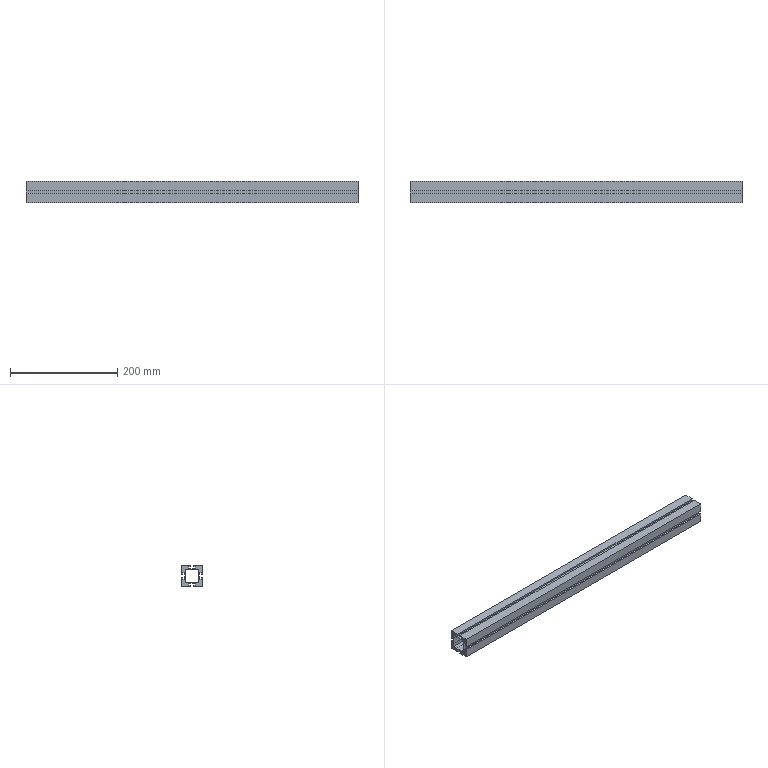Part | SolidWorks | features Extrusion 1 | 1 solid | 42 faces | box 620 x 40 x 40 mm | volume 431520 mm3 | plane 42
STEP:
#1=CARTESIAN_POINT('',(620.,3.,-20.));
#2=VERTEX_POINT('',#1);
#3=CARTESIAN_POINT('',(620.,20.,-20.));
#4=VERTEX_POINT('',#3);
#5=CARTESIAN_POINT('',(620.,3.,-20.));
#6=DIRECTION('',(0.,1.,0.));
#7=VECTOR('',#6,1000.);
#8=LINE('',#5,#7);
#9=EDGE_CURVE('',#2,#4,#8,.T.);
#10=ORIENTED_EDGE('',*,*,#9,.T.);
#11=CARTESIAN_POINT('',(620.,20.,-3.));
#12=VERTEX_POINT('',#11);
#13=CARTESIAN_POINT('',(620.,20.,-3.));
#14=DIRECTION('',(0.,0.,1.));
#15=VECTOR('',#14,1000.);
#16=LINE('',#13,#15);
#17=EDGE_CURVE('',#4,#12,#16,.T.);
#18=ORIENTED_EDGE('',*,*,#17,.T.);
#19=CARTESIAN_POINT('',(620.,17.,-3.));
#20=VERTEX_POINT('',#19);
#21=CARTESIAN_POINT('',(620.,20.,-3.));
#22=DIRECTION('',(0.,-1.,0.));
#23=VECTOR('',#22,1000.);
#24=LINE('',#21,#23);
#25=EDGE_CURVE('',#12,#20,#24,.T.);
#26=ORIENTED_EDGE('',*,*,#25,.T.);
#27=CARTESIAN_POINT('',(620.,17.,-6.5));
#28=VERTEX_POINT('',#27);
#29=CARTESIAN_POINT('',(620.,17.,-3.));
#30=DIRECTION('',(0.,0.,-1.));
#31=VECTOR('',#30,1000.);
#32=LINE('',#29,#31);
#33=EDGE_CURVE('',#20,#28,#32,.T.);
#34=ORIENTED_EDGE('',*,*,#33,.T.);
#35=CARTESIAN_POINT('',(620.,14.,-6.5));
#36=VERTEX_POINT('',#35);
#37=CARTESIAN_POINT('',(620.,17.,-6.5));
#38=DIRECTION('',(0.,-1.,0.));
#39=VECTOR('',#38,1000.);
#40=LINE('',#37,#39);
#41=EDGE_CURVE('',#28,#36,#40,.T.);
#42=ORIENTED_EDGE('',*,*,#41,.T.);
#43=CARTESIAN_POINT('',(620.,14.,6.5));
#44=VERTEX_POINT('',#43);
#45=CARTESIAN_POINT('',(620.,14.,6.5));
#46=DIRECTION('',(0.,0.,1.));
#47=VECTOR('',#46,1000.);
#48=LINE('',#45,#47);
#49=EDGE_CURVE('',#36,#44,#48,.T.);
#50=ORIENTED_EDGE('',*,*,#49,.T.);
#51=CARTESIAN_POINT('',(620.,17.,6.5));
#52=VERTEX_POINT('',#51);
#53=CARTESIAN_POINT('',(620.,17.,6.5));
#54=DIRECTION('',(0.,1.,0.));
#55=VECTOR('',#54,1000.);
#56=LINE('',#53,#55);
#57=EDGE_CURVE('',#44,#52,#56,.T.);
#58=ORIENTED_EDGE('',*,*,#57,.T.);
#59=CARTESIAN_POINT('',(620.,17.,3.));
#60=VERTEX_POINT('',#59);
#61=CARTESIAN_POINT('',(620.,17.,6.5));
#62=DIRECTION('',(0.,0.,-1.));
#63=VECTOR('',#62,1000.);
#64=LINE('',#61,#63);
#65=EDGE_CURVE('',#52,#60,#64,.T.);
#66=ORIENTED_EDGE('',*,*,#65,.T.);
#67=CARTESIAN_POINT('',(620.,20.,3.));
#68=VERTEX_POINT('',#67);
#69=CARTESIAN_POINT('',(620.,20.,3.));
#70=DIRECTION('',(0.,1.,0.));
#71=VECTOR('',#70,1000.);
#72=LINE('',#69,#71);
#73=EDGE_CURVE('',#60,#68,#72,.T.);
#74=ORIENTED_EDGE('',*,*,#73,.T.);
#75=CARTESIAN_POINT('',(620.,20.,20.));
#76=VERTEX_POINT('',#75);
#77=CARTESIAN_POINT('',(620.,20.,20.));
#78=DIRECTION('',(0.,0.,1.));
#79=VECTOR('',#78,1000.);
#80=LINE('',#77,#79);
#81=EDGE_CURVE('',#68,#76,#80,.T.);
#82=ORIENTED_EDGE('',*,*,#81,.T.);
#83=CARTESIAN_POINT('',(620.,3.,20.));
#84=VERTEX_POINT('',#83);
#85=CARTESIAN_POINT('',(620.,3.,20.));
#86=DIRECTION('',(0.,-1.,0.));
#87=VECTOR('',#86,1000.);
#88=LINE('',#85,#87);
#89=EDGE_CURVE('',#76,#84,#88,.T.);
#90=ORIENTED_EDGE('',*,*,#89,.T.);
#91=CARTESIAN_POINT('',(620.,3.,17.));
#92=VERTEX_POINT('',#91);
#93=CARTESIAN_POINT('',(620.,3.,17.));
#94=DIRECTION('',(0.,0.,-1.));
#95=VECTOR('',#94,1000.);
#96=LINE('',#93,#95);
#97=EDGE_CURVE('',#84,#92,#96,.T.);
#98=ORIENTED_EDGE('',*,*,#97,.T.);
#99=CARTESIAN_POINT('',(620.,6.5,17.));
#100=VERTEX_POINT('',#99);
#101=CARTESIAN_POINT('',(620.,3.,17.));
#102=DIRECTION('',(0.,1.,0.));
#103=VECTOR('',#102,1000.);
#104=LINE('',#101,#103);
#105=EDGE_CURVE('',#92,#100,#104,.T.);
#106=ORIENTED_EDGE('',*,*,#105,.T.);
#107=CARTESIAN_POINT('',(620.,6.5,14.));
#108=VERTEX_POINT('',#107);
#109=CARTESIAN_POINT('',(620.,6.5,14.));
#110=DIRECTION('',(0.,0.,-1.));
#111=VECTOR('',#110,1000.);
#112=LINE('',#109,#111);
#113=EDGE_CURVE('',#100,#108,#112,.T.);
#114=ORIENTED_EDGE('',*,*,#113,.T.);
#115=CARTESIAN_POINT('',(620.,-6.5,14.));
#116=VERTEX_POINT('',#115);
#117=CARTESIAN_POINT('',(620.,-6.5,14.));
#118=DIRECTION('',(0.,-1.,0.));
#119=VECTOR('',#118,1000.);
#120=LINE('',#117,#119);
#121=EDGE_CURVE('',#108,#116,#120,.T.);
#122=ORIENTED_EDGE('',*,*,#121,.T.);
#123=CARTESIAN_POINT('',(620.,-6.5,17.));
#124=VERTEX_POINT('',#123);
#125=CARTESIAN_POINT('',(620.,-6.5,14.));
#126=DIRECTION('',(0.,0.,1.));
#127=VECTOR('',#126,1000.);
#128=LINE('',#125,#127);
#129=EDGE_CURVE('',#116,#124,#128,.T.);
#130=ORIENTED_EDGE('',*,*,#129,.T.);
#131=CARTESIAN_POINT('',(620.,-3.,17.));
#132=VERTEX_POINT('',#131);
#133=CARTESIAN_POINT('',(620.,-6.5,17.));
#134=DIRECTION('',(0.,1.,0.));
#135=VECTOR('',#134,1000.);
#136=LINE('',#133,#135);
#137=EDGE_CURVE('',#124,#132,#136,.T.);
#138=ORIENTED_EDGE('',*,*,#137,.T.);
#139=CARTESIAN_POINT('',(620.,-3.,20.));
#140=VERTEX_POINT('',#139);
#141=CARTESIAN_POINT('',(620.,-3.,17.));
#142=DIRECTION('',(0.,0.,1.));
#143=VECTOR('',#142,1000.);
#144=LINE('',#141,#143);
#145=EDGE_CURVE('',#132,#140,#144,.T.);
#146=ORIENTED_EDGE('',*,*,#145,.T.);
#147=CARTESIAN_POINT('',(620.,-20.,20.));
#148=VERTEX_POINT('',#147);
#149=CARTESIAN_POINT('',(620.,-20.,20.));
#150=DIRECTION('',(0.,-1.,0.));
#151=VECTOR('',#150,1000.);
#152=LINE('',#149,#151);
#153=EDGE_CURVE('',#140,#148,#152,.T.);
#154=ORIENTED_EDGE('',*,*,#153,.T.);
#155=CARTESIAN_POINT('',(620.,-20.,3.));
#156=VERTEX_POINT('',#155);
#157=CARTESIAN_POINT('',(620.,-20.,20.));
#158=DIRECTION('',(0.,0.,-1.));
#159=VECTOR('',#158,1000.);
#160=LINE('',#157,#159);
#161=EDGE_CURVE('',#148,#156,#160,.T.);
#162=ORIENTED_EDGE('',*,*,#161,.T.);
#163=CARTESIAN_POINT('',(620.,-17.,3.));
#164=VERTEX_POINT('',#163);
#165=CARTESIAN_POINT('',(620.,-20.,3.));
#166=DIRECTION('',(0.,1.,0.));
#167=VECTOR('',#166,1000.);
#168=LINE('',#165,#167);
#169=EDGE_CURVE('',#156,#164,#168,.T.);
#170=ORIENTED_EDGE('',*,*,#169,.T.);
#171=CARTESIAN_POINT('',(620.,-17.,6.5));
#172=VERTEX_POINT('',#171);
#173=CARTESIAN_POINT('',(620.,-17.,6.5));
#174=DIRECTION('',(0.,0.,1.));
#175=VECTOR('',#174,1000.);
#176=LINE('',#173,#175);
#177=EDGE_CURVE('',#164,#172,#176,.T.);
#178=ORIENTED_EDGE('',*,*,#177,.T.);
#179=CARTESIAN_POINT('',(620.,-14.,6.5));
#180=VERTEX_POINT('',#179);
#181=CARTESIAN_POINT('',(620.,-17.,6.5));
#182=DIRECTION('',(0.,1.,0.));
#183=VECTOR('',#182,1000.);
#184=LINE('',#181,#183);
#185=EDGE_CURVE('',#172,#180,#184,.T.);
#186=ORIENTED_EDGE('',*,*,#185,.T.);
#187=CARTESIAN_POINT('',(620.,-14.,-6.5));
#188=VERTEX_POINT('',#187);
#189=CARTESIAN_POINT('',(620.,-14.,6.5));
#190=DIRECTION('',(0.,0.,-1.));
#191=VECTOR('',#190,1000.);
#192=LINE('',#189,#191);
#193=EDGE_CURVE('',#180,#188,#192,.T.);
#194=ORIENTED_EDGE('',*,*,#193,.T.);
#195=CARTESIAN_POINT('',(620.,-17.,-6.5));
#196=VERTEX_POINT('',#195);
#197=CARTESIAN_POINT('',(620.,-17.,-6.5));
#198=DIRECTION('',(0.,-1.,0.));
#199=VECTOR('',#198,1000.);
#200=LINE('',#197,#199);
#201=EDGE_CURVE('',#188,#196,#200,.T.);
#202=ORIENTED_EDGE('',*,*,#201,.T.);
#203=CARTESIAN_POINT('',(620.,-17.,-3.));
#204=VERTEX_POINT('',#203);
#205=CARTESIAN_POINT('',(620.,-17.,-3.));
#206=DIRECTION('',(0.,0.,1.));
#207=VECTOR('',#206,1000.);
#208=LINE('',#205,#207);
#209=EDGE_CURVE('',#196,#204,#208,.T.);
#210=ORIENTED_EDGE('',*,*,#209,.T.);
#211=CARTESIAN_POINT('',(620.,-20.,-3.));
#212=VERTEX_POINT('',#211);
#213=CARTESIAN_POINT('',(620.,-20.,-3.));
#214=DIRECTION('',(0.,-1.,0.));
#215=VECTOR('',#214,1000.);
#216=LINE('',#213,#215);
#217=EDGE_CURVE('',#204,#212,#216,.T.);
#218=ORIENTED_EDGE('',*,*,#217,.T.);
#219=CARTESIAN_POINT('',(620.,-20.,-20.));
#220=VERTEX_POINT('',#219);
#221=CARTESIAN_POINT('',(620.,-20.,-3.));
#222=DIRECTION('',(0.,0.,-1.));
#223=VECTOR('',#222,1000.);
#224=LINE('',#221,#223);
#225=EDGE_CURVE('',#212,#220,#224,.T.);
#226=ORIENTED_EDGE('',*,*,#225,.T.);
#227=CARTESIAN_POINT('',(620.,-3.,-20.));
#228=VERTEX_POINT('',#227);
#229=CARTESIAN_POINT('',(620.,-20.,-20.));
#230=DIRECTION('',(0.,1.,0.));
#231=VECTOR('',#230,1000.);
#232=LINE('',#229,#231);
#233=EDGE_CURVE('',#220,#228,#232,.T.);
#234=ORIENTED_EDGE('',*,*,#233,.T.);
#235=CARTESIAN_POINT('',(620.,-3.,-17.));
#236=VERTEX_POINT('',#235);
#237=CARTESIAN_POINT('',(620.,-3.,-17.));
#238=DIRECTION('',(0.,0.,1.));
#239=VECTOR('',#238,1000.);
#240=LINE('',#237,#239);
#241=EDGE_CURVE('',#228,#236,#240,.T.);
#242=ORIENTED_EDGE('',*,*,#241,.T.);
#243=CARTESIAN_POINT('',(620.,-6.5,-17.));
#244=VERTEX_POINT('',#243);
#245=CARTESIAN_POINT('',(620.,-6.5,-17.));
#246=DIRECTION('',(0.,-1.,0.));
#247=VECTOR('',#246,1000.);
#248=LINE('',#245,#247);
#249=EDGE_CURVE('',#236,#244,#248,.T.);
#250=ORIENTED_EDGE('',*,*,#249,.T.);
#251=CARTESIAN_POINT('',(620.,-6.5,-14.));
#252=VERTEX_POINT('',#251);
#253=CARTESIAN_POINT('',(620.,-6.5,-14.));
#254=DIRECTION('',(0.,0.,1.));
#255=VECTOR('',#254,1000.);
#256=LINE('',#253,#255);
#257=EDGE_CURVE('',#244,#252,#256,.T.);
#258=ORIENTED_EDGE('',*,*,#257,.T.);
#259=CARTESIAN_POINT('',(620.,6.5,-14.));
#260=VERTEX_POINT('',#259);
#261=CARTESIAN_POINT('',(620.,-6.5,-14.));
#262=DIRECTION('',(0.,1.,0.));
#263=VECTOR('',#262,1000.);
#264=LINE('',#261,#263);
#265=EDGE_CURVE('',#252,#260,#264,.T.);
#266=ORIENTED_EDGE('',*,*,#265,.T.);
#267=CARTESIAN_POINT('',(620.,6.5,-17.));
#268=VERTEX_POINT('',#267);
#269=CARTESIAN_POINT('',(620.,6.5,-14.));
#270=DIRECTION('',(0.,0.,-1.));
#271=VECTOR('',#270,1000.);
#272=LINE('',#269,#271);
#273=EDGE_CURVE('',#260,#268,#272,.T.);
#274=ORIENTED_EDGE('',*,*,#273,.T.);
#275=CARTESIAN_POINT('',(620.,3.,-17.));
#276=VERTEX_POINT('',#275);
#277=CARTESIAN_POINT('',(620.,3.,-17.));
#278=DIRECTION('',(0.,-1.,0.));
#279=VECTOR('',#278,1000.);
#280=LINE('',#277,#279);
#281=EDGE_CURVE('',#268,#276,#280,.T.);
#282=ORIENTED_EDGE('',*,*,#281,.T.);
#283=CARTESIAN_POINT('',(620.,3.,-17.));
#284=DIRECTION('',(0.,0.,-1.));
#285=VECTOR('',#284,1000.);
#286=LINE('',#283,#285);
#287=EDGE_CURVE('',#276,#2,#286,.T.);
#288=ORIENTED_EDGE('',*,*,#287,.T.);
#289=EDGE_LOOP('',(#10,#18,#26,#34,#42,#50,#58,#66,#74,#82,#90,#98,#106,#114,#122,#130,#138,#146,#154,#162,#170,#178,#186,#194,#202,#210,#218,#226,#234,#242,#250,#258,#266,#274,#282,#288));
#290=FACE_OUTER_BOUND('',#289,.T.);
#291=CARTESIAN_POINT('',(620.,-13.,-13.));
#292=VERTEX_POINT('',#291);
#293=CARTESIAN_POINT('',(620.,13.,-13.));
#294=VERTEX_POINT('',#293);
#295=CARTESIAN_POINT('',(620.,-13.,-13.));
#296=DIRECTION('',(0.,1.,0.));
#297=VECTOR('',#296,1000.);
#298=LINE('',#295,#297);
#299=EDGE_CURVE('',#292,#294,#298,.T.);
#300=ORIENTED_EDGE('',*,*,#299,.F.);
#301=CARTESIAN_POINT('',(620.,-13.,13.));
#302=VERTEX_POINT('',#301);
#303=CARTESIAN_POINT('',(620.,-13.,13.));
#304=DIRECTION('',(0.,0.,-1.));
#305=VECTOR('',#304,1000.);
#306=LINE('',#303,#305);
#307=EDGE_CURVE('',#302,#292,#306,.T.);
#308=ORIENTED_EDGE('',*,*,#307,.F.);
#309=CARTESIAN_POINT('',(620.,13.,13.));
#310=VERTEX_POINT('',#309);
#311=CARTESIAN_POINT('',(620.,-13.,13.));
#312=DIRECTION('',(0.,-1.,0.));
#313=VECTOR('',#312,1000.);
#314=LINE('',#311,#313);
#315=EDGE_CURVE('',#310,#302,#314,.T.);
#316=ORIENTED_EDGE('',*,*,#315,.F.);
#317=CARTESIAN_POINT('',(620.,13.,13.));
#318=DIRECTION('',(0.,0.,1.));
#319=VECTOR('',#318,1000.);
#320=LINE('',#317,#319);
#321=EDGE_CURVE('',#294,#310,#320,.T.);
#322=ORIENTED_EDGE('',*,*,#321,.F.);
#323=EDGE_LOOP('',(#300,#308,#316,#322));
#324=FACE_BOUND('',#323,.T.);
#325=CARTESIAN_POINT('',(620.,20.,-20.));
#326=DIRECTION('',(-1.,0.,0.));
#327=DIRECTION('',(0.,0.,1.));
#328=AXIS2_PLACEMENT_3D('',#325,#326,#327);
#329=PLANE('',#328);
#330=ADVANCED_FACE('',(#290,#324),#329,.F.);
#331=CARTESIAN_POINT('',(0.,3.,-20.));
#332=VERTEX_POINT('',#331);
#333=CARTESIAN_POINT('',(0.,20.,-20.));
#334=VERTEX_POINT('',#333);
#335=CARTESIAN_POINT('',(0.,3.,-20.));
#336=DIRECTION('',(0.,1.,0.));
#337=VECTOR('',#336,1000.);
#338=LINE('',#335,#337);
#339=EDGE_CURVE('',#332,#334,#338,.T.);
#340=ORIENTED_EDGE('',*,*,#339,.F.);
#341=CARTESIAN_POINT('',(0.,3.,-17.));
#342=VERTEX_POINT('',#341);
#343=CARTESIAN_POINT('',(0.,3.,-17.));
#344=DIRECTION('',(0.,0.,-1.));
#345=VECTOR('',#344,1000.);
#346=LINE('',#343,#345);
#347=EDGE_CURVE('',#342,#332,#346,.T.);
#348=ORIENTED_EDGE('',*,*,#347,.F.);
#349=CARTESIAN_POINT('',(0.,6.5,-17.));
#350=VERTEX_POINT('',#349);
#351=CARTESIAN_POINT('',(0.,3.,-17.));
#352=DIRECTION('',(0.,-1.,0.));
#353=VECTOR('',#352,1000.);
#354=LINE('',#351,#353);
#355=EDGE_CURVE('',#350,#342,#354,.T.);
#356=ORIENTED_EDGE('',*,*,#355,.F.);
#357=CARTESIAN_POINT('',(0.,6.5,-14.));
#358=VERTEX_POINT('',#357);
#359=CARTESIAN_POINT('',(0.,6.5,-14.));
#360=DIRECTION('',(0.,0.,-1.));
#361=VECTOR('',#360,1000.);
#362=LINE('',#359,#361);
#363=EDGE_CURVE('',#358,#350,#362,.T.);
#364=ORIENTED_EDGE('',*,*,#363,.F.);
#365=CARTESIAN_POINT('',(0.,-6.5,-14.));
#366=VERTEX_POINT('',#365);
#367=CARTESIAN_POINT('',(0.,-6.5,-14.));
#368=DIRECTION('',(0.,1.,0.));
#369=VECTOR('',#368,1000.);
#370=LINE('',#367,#369);
#371=EDGE_CURVE('',#366,#358,#370,.T.);
#372=ORIENTED_EDGE('',*,*,#371,.F.);
#373=CARTESIAN_POINT('',(0.,-6.5,-17.));
#374=VERTEX_POINT('',#373);
#375=CARTESIAN_POINT('',(0.,-6.5,-14.));
#376=DIRECTION('',(0.,0.,1.));
#377=VECTOR('',#376,1000.);
#378=LINE('',#375,#377);
#379=EDGE_CURVE('',#374,#366,#378,.T.);
#380=ORIENTED_EDGE('',*,*,#379,.F.);
#381=CARTESIAN_POINT('',(0.,-3.,-17.));
#382=VERTEX_POINT('',#381);
#383=CARTESIAN_POINT('',(0.,-6.5,-17.));
#384=DIRECTION('',(0.,-1.,0.));
#385=VECTOR('',#384,1000.);
#386=LINE('',#383,#385);
#387=EDGE_CURVE('',#382,#374,#386,.T.);
#388=ORIENTED_EDGE('',*,*,#387,.F.);
#389=CARTESIAN_POINT('',(0.,-3.,-20.));
#390=VERTEX_POINT('',#389);
#391=CARTESIAN_POINT('',(0.,-3.,-17.));
#392=DIRECTION('',(0.,0.,1.));
#393=VECTOR('',#392,1000.);
#394=LINE('',#391,#393);
#395=EDGE_CURVE('',#390,#382,#394,.T.);
#396=ORIENTED_EDGE('',*,*,#395,.F.);
#397=CARTESIAN_POINT('',(0.,-20.,-20.));
#398=VERTEX_POINT('',#397);
#399=CARTESIAN_POINT('',(0.,-20.,-20.));
#400=DIRECTION('',(0.,1.,0.));
#401=VECTOR('',#400,1000.);
#402=LINE('',#399,#401);
#403=EDGE_CURVE('',#398,#390,#402,.T.);
#404=ORIENTED_EDGE('',*,*,#403,.F.);
#405=CARTESIAN_POINT('',(0.,-20.,-3.));
#406=VERTEX_POINT('',#405);
#407=CARTESIAN_POINT('',(0.,-20.,-3.));
#408=DIRECTION('',(0.,0.,-1.));
#409=VECTOR('',#408,1000.);
#410=LINE('',#407,#409);
#411=EDGE_CURVE('',#406,#398,#410,.T.);
#412=ORIENTED_EDGE('',*,*,#411,.F.);
#413=CARTESIAN_POINT('',(0.,-17.,-3.));
#414=VERTEX_POINT('',#413);
#415=CARTESIAN_POINT('',(0.,-20.,-3.));
#416=DIRECTION('',(0.,-1.,0.));
#417=VECTOR('',#416,1000.);
#418=LINE('',#415,#417);
#419=EDGE_CURVE('',#414,#406,#418,.T.);
#420=ORIENTED_EDGE('',*,*,#419,.F.);
#421=CARTESIAN_POINT('',(0.,-17.,-6.5));
#422=VERTEX_POINT('',#421);
#423=CARTESIAN_POINT('',(0.,-17.,-3.));
#424=DIRECTION('',(0.,0.,1.));
#425=VECTOR('',#424,1000.);
#426=LINE('',#423,#425);
#427=EDGE_CURVE('',#422,#414,#426,.T.);
#428=ORIENTED_EDGE('',*,*,#427,.F.);
#429=CARTESIAN_POINT('',(0.,-14.,-6.5));
#430=VERTEX_POINT('',#429);
#431=CARTESIAN_POINT('',(0.,-17.,-6.5));
#432=DIRECTION('',(0.,-1.,0.));
#433=VECTOR('',#432,1000.);
#434=LINE('',#431,#433);
#435=EDGE_CURVE('',#430,#422,#434,.T.);
#436=ORIENTED_EDGE('',*,*,#435,.F.);
#437=CARTESIAN_POINT('',(0.,-14.,6.5));
#438=VERTEX_POINT('',#437);
#439=CARTESIAN_POINT('',(0.,-14.,6.5));
#440=DIRECTION('',(0.,0.,-1.));
#441=VECTOR('',#440,1000.);
#442=LINE('',#439,#441);
#443=EDGE_CURVE('',#438,#430,#442,.T.);
#444=ORIENTED_EDGE('',*,*,#443,.F.);
#445=CARTESIAN_POINT('',(0.,-17.,6.5));
#446=VERTEX_POINT('',#445);
#447=CARTESIAN_POINT('',(0.,-17.,6.5));
#448=DIRECTION('',(0.,1.,0.));
#449=VECTOR('',#448,1000.);
#450=LINE('',#447,#449);
#451=EDGE_CURVE('',#446,#438,#450,.T.);
#452=ORIENTED_EDGE('',*,*,#451,.F.);
#453=CARTESIAN_POINT('',(0.,-17.,3.));
#454=VERTEX_POINT('',#453);
#455=CARTESIAN_POINT('',(0.,-17.,6.5));
#456=DIRECTION('',(0.,0.,1.));
#457=VECTOR('',#456,1000.);
#458=LINE('',#455,#457);
#459=EDGE_CURVE('',#454,#446,#458,.T.);
#460=ORIENTED_EDGE('',*,*,#459,.F.);
#461=CARTESIAN_POINT('',(0.,-20.,3.));
#462=VERTEX_POINT('',#461);
#463=CARTESIAN_POINT('',(0.,-20.,3.));
#464=DIRECTION('',(0.,1.,0.));
#465=VECTOR('',#464,1000.);
#466=LINE('',#463,#465);
#467=EDGE_CURVE('',#462,#454,#466,.T.);
#468=ORIENTED_EDGE('',*,*,#467,.F.);
#469=CARTESIAN_POINT('',(0.,-20.,20.));
#470=VERTEX_POINT('',#469);
#471=CARTESIAN_POINT('',(0.,-20.,20.));
#472=DIRECTION('',(0.,0.,-1.));
#473=VECTOR('',#472,1000.);
#474=LINE('',#471,#473);
#475=EDGE_CURVE('',#470,#462,#474,.T.);
#476=ORIENTED_EDGE('',*,*,#475,.F.);
#477=CARTESIAN_POINT('',(0.,-3.,20.));
#478=VERTEX_POINT('',#477);
#479=CARTESIAN_POINT('',(0.,-20.,20.));
#480=DIRECTION('',(0.,-1.,0.));
#481=VECTOR('',#480,1000.);
#482=LINE('',#479,#481);
#483=EDGE_CURVE('',#478,#470,#482,.T.);
#484=ORIENTED_EDGE('',*,*,#483,.F.);
#485=CARTESIAN_POINT('',(0.,-3.,17.));
#486=VERTEX_POINT('',#485);
#487=CARTESIAN_POINT('',(0.,-3.,17.));
#488=DIRECTION('',(0.,0.,1.));
#489=VECTOR('',#488,1000.);
#490=LINE('',#487,#489);
#491=EDGE_CURVE('',#486,#478,#490,.T.);
#492=ORIENTED_EDGE('',*,*,#491,.F.);
#493=CARTESIAN_POINT('',(0.,-6.5,17.));
#494=VERTEX_POINT('',#493);
#495=CARTESIAN_POINT('',(0.,-6.5,17.));
#496=DIRECTION('',(0.,1.,0.));
#497=VECTOR('',#496,1000.);
#498=LINE('',#495,#497);
#499=EDGE_CURVE('',#494,#486,#498,.T.);
#500=ORIENTED_EDGE('',*,*,#499,.F.);
#501=CARTESIAN_POINT('',(0.,-6.5,14.));
#502=VERTEX_POINT('',#501);
#503=CARTESIAN_POINT('',(0.,-6.5,14.));
#504=DIRECTION('',(0.,0.,1.));
#505=VECTOR('',#504,1000.);
#506=LINE('',#503,#505);
#507=EDGE_CURVE('',#502,#494,#506,.T.);
#508=ORIENTED_EDGE('',*,*,#507,.F.);
#509=CARTESIAN_POINT('',(0.,6.5,14.));
#510=VERTEX_POINT('',#509);
#511=CARTESIAN_POINT('',(0.,-6.5,14.));
#512=DIRECTION('',(0.,-1.,0.));
#513=VECTOR('',#512,1000.);
#514=LINE('',#511,#513);
#515=EDGE_CURVE('',#510,#502,#514,.T.);
#516=ORIENTED_EDGE('',*,*,#515,.F.);
#517=CARTESIAN_POINT('',(0.,6.5,17.));
#518=VERTEX_POINT('',#517);
#519=CARTESIAN_POINT('',(0.,6.5,14.));
#520=DIRECTION('',(0.,0.,-1.));
#521=VECTOR('',#520,1000.);
#522=LINE('',#519,#521);
#523=EDGE_CURVE('',#518,#510,#522,.T.);
#524=ORIENTED_EDGE('',*,*,#523,.F.);
#525=CARTESIAN_POINT('',(0.,3.,17.));
#526=VERTEX_POINT('',#525);
#527=CARTESIAN_POINT('',(0.,3.,17.));
#528=DIRECTION('',(0.,1.,0.));
#529=VECTOR('',#528,1000.);
#530=LINE('',#527,#529);
#531=EDGE_CURVE('',#526,#518,#530,.T.);
#532=ORIENTED_EDGE('',*,*,#531,.F.);
#533=CARTESIAN_POINT('',(0.,3.,20.));
#534=VERTEX_POINT('',#533);
#535=CARTESIAN_POINT('',(0.,3.,17.));
#536=DIRECTION('',(0.,0.,-1.));
#537=VECTOR('',#536,1000.);
#538=LINE('',#535,#537);
#539=EDGE_CURVE('',#534,#526,#538,.T.);
#540=ORIENTED_EDGE('',*,*,#539,.F.);
#541=CARTESIAN_POINT('',(0.,20.,20.));
#542=VERTEX_POINT('',#541);
#543=CARTESIAN_POINT('',(0.,3.,20.));
#544=DIRECTION('',(0.,-1.,0.));
#545=VECTOR('',#544,1000.);
#546=LINE('',#543,#545);
#547=EDGE_CURVE('',#542,#534,#546,.T.);
#548=ORIENTED_EDGE('',*,*,#547,.F.);
#549=CARTESIAN_POINT('',(0.,20.,3.));
#550=VERTEX_POINT('',#549);
#551=CARTESIAN_POINT('',(0.,20.,20.));
#552=DIRECTION('',(0.,0.,1.));
#553=VECTOR('',#552,1000.);
#554=LINE('',#551,#553);
#555=EDGE_CURVE('',#550,#542,#554,.T.);
#556=ORIENTED_EDGE('',*,*,#555,.F.);
#557=CARTESIAN_POINT('',(0.,17.,3.));
#558=VERTEX_POINT('',#557);
#559=CARTESIAN_POINT('',(0.,20.,3.));
#560=DIRECTION('',(0.,1.,0.));
#561=VECTOR('',#560,1000.);
#562=LINE('',#559,#561);
#563=EDGE_CURVE('',#558,#550,#562,.T.);
#564=ORIENTED_EDGE('',*,*,#563,.F.);
#565=CARTESIAN_POINT('',(0.,17.,6.5));
#566=VERTEX_POINT('',#565);
#567=CARTESIAN_POINT('',(0.,17.,6.5));
#568=DIRECTION('',(0.,0.,-1.));
#569=VECTOR('',#568,1000.);
#570=LINE('',#567,#569);
#571=EDGE_CURVE('',#566,#558,#570,.T.);
#572=ORIENTED_EDGE('',*,*,#571,.F.);
#573=CARTESIAN_POINT('',(0.,14.,6.5));
#574=VERTEX_POINT('',#573);
#575=CARTESIAN_POINT('',(0.,17.,6.5));
#576=DIRECTION('',(0.,1.,0.));
#577=VECTOR('',#576,1000.);
#578=LINE('',#575,#577);
#579=EDGE_CURVE('',#574,#566,#578,.T.);
#580=ORIENTED_EDGE('',*,*,#579,.F.);
#581=CARTESIAN_POINT('',(0.,14.,-6.5));
#582=VERTEX_POINT('',#581);
#583=CARTESIAN_POINT('',(0.,14.,6.5));
#584=DIRECTION('',(0.,0.,1.));
#585=VECTOR('',#584,1000.);
#586=LINE('',#583,#585);
#587=EDGE_CURVE('',#582,#574,#586,.T.);
#588=ORIENTED_EDGE('',*,*,#587,.F.);
#589=CARTESIAN_POINT('',(0.,17.,-6.5));
#590=VERTEX_POINT('',#589);
#591=CARTESIAN_POINT('',(0.,17.,-6.5));
#592=DIRECTION('',(0.,-1.,0.));
#593=VECTOR('',#592,1000.);
#594=LINE('',#591,#593);
#595=EDGE_CURVE('',#590,#582,#594,.T.);
#596=ORIENTED_EDGE('',*,*,#595,.F.);
#597=CARTESIAN_POINT('',(0.,17.,-3.));
#598=VERTEX_POINT('',#597);
#599=CARTESIAN_POINT('',(0.,17.,-3.));
#600=DIRECTION('',(0.,0.,-1.));
#601=VECTOR('',#600,1000.);
#602=LINE('',#599,#601);
#603=EDGE_CURVE('',#598,#590,#602,.T.);
#604=ORIENTED_EDGE('',*,*,#603,.F.);
#605=CARTESIAN_POINT('',(0.,20.,-3.));
#606=VERTEX_POINT('',#605);
#607=CARTESIAN_POINT('',(0.,20.,-3.));
#608=DIRECTION('',(0.,-1.,0.));
#609=VECTOR('',#608,1000.);
#610=LINE('',#607,#609);
#611=EDGE_CURVE('',#606,#598,#610,.T.);
#612=ORIENTED_EDGE('',*,*,#611,.F.);
#613=CARTESIAN_POINT('',(0.,20.,-3.));
#614=DIRECTION('',(0.,0.,1.));
#615=VECTOR('',#614,1000.);
#616=LINE('',#613,#615);
#617=EDGE_CURVE('',#334,#606,#616,.T.);
#618=ORIENTED_EDGE('',*,*,#617,.F.);
#619=EDGE_LOOP('',(#340,#348,#356,#364,#372,#380,#388,#396,#404,#412,#420,#428,#436,#444,#452,#460,#468,#476,#484,#492,#500,#508,#516,#524,#532,#540,#548,#556,#564,#572,#580,#588,#596,#604,#612,#618));
#620=FACE_OUTER_BOUND('',#619,.T.);
#621=CARTESIAN_POINT('',(0.,-13.,13.));
#622=VERTEX_POINT('',#621);
#623=CARTESIAN_POINT('',(0.,-13.,-13.));
#624=VERTEX_POINT('',#623);
#625=CARTESIAN_POINT('',(0.,-13.,13.));
#626=DIRECTION('',(0.,0.,-1.));
#627=VECTOR('',#626,1000.);
#628=LINE('',#625,#627);
#629=EDGE_CURVE('',#622,#624,#628,.T.);
#630=ORIENTED_EDGE('',*,*,#629,.T.);
#631=CARTESIAN_POINT('',(0.,13.,-13.));
#632=VERTEX_POINT('',#631);
#633=CARTESIAN_POINT('',(0.,-13.,-13.));
#634=DIRECTION('',(0.,1.,0.));
#635=VECTOR('',#634,1000.);
#636=LINE('',#633,#635);
#637=EDGE_CURVE('',#624,#632,#636,.T.);
#638=ORIENTED_EDGE('',*,*,#637,.T.);
#639=CARTESIAN_POINT('',(0.,13.,13.));
#640=VERTEX_POINT('',#639);
#641=CARTESIAN_POINT('',(0.,13.,13.));
#642=DIRECTION('',(0.,0.,1.));
#643=VECTOR('',#642,1000.);
#644=LINE('',#641,#643);
#645=EDGE_CURVE('',#632,#640,#644,.T.);
#646=ORIENTED_EDGE('',*,*,#645,.T.);
#647=CARTESIAN_POINT('',(0.,-13.,13.));
#648=DIRECTION('',(0.,-1.,0.));
#649=VECTOR('',#648,1000.);
#650=LINE('',#647,#649);
#651=EDGE_CURVE('',#640,#622,#650,.T.);
#652=ORIENTED_EDGE('',*,*,#651,.T.);
#653=EDGE_LOOP('',(#630,#638,#646,#652));
#654=FACE_BOUND('',#653,.T.);
#655=CARTESIAN_POINT('',(0.,20.,-20.));
#656=DIRECTION('',(-1.,0.,0.));
#657=DIRECTION('',(0.,0.,1.));
#658=AXIS2_PLACEMENT_3D('',#655,#656,#657);
#659=PLANE('',#658);
#660=ADVANCED_FACE('',(#620,#654),#659,.T.);
#661=ORIENTED_EDGE('',*,*,#339,.T.);
#662=CARTESIAN_POINT('',(620.,20.,-20.));
#663=DIRECTION('',(-1.,0.,0.));
#664=VECTOR('',#663,1000.);
#665=LINE('',#662,#664);
#666=EDGE_CURVE('',#4,#334,#665,.T.);
#667=ORIENTED_EDGE('',*,*,#666,.F.);
#668=ORIENTED_EDGE('',*,*,#9,.F.);
#669=CARTESIAN_POINT('',(620.,3.,-20.));
#670=DIRECTION('',(-1.,0.,0.));
#671=VECTOR('',#670,1000.);
#672=LINE('',#669,#671);
#673=EDGE_CURVE('',#2,#332,#672,.T.);
#674=ORIENTED_EDGE('',*,*,#673,.T.);
#675=EDGE_LOOP('',(#661,#667,#668,#674));
#676=FACE_OUTER_BOUND('',#675,.T.);
#677=CARTESIAN_POINT('',(620.,3.,-20.));
#678=DIRECTION('',(0.,0.,1.));
#679=DIRECTION('',(0.,-1.,0.));
#680=AXIS2_PLACEMENT_3D('',#677,#678,#679);
#681=PLANE('',#680);
#682=ADVANCED_FACE('',(#676),#681,.F.);
#683=ORIENTED_EDGE('',*,*,#617,.T.);
#684=CARTESIAN_POINT('',(620.,20.,-3.));
#685=DIRECTION('',(-1.,0.,0.));
#686=VECTOR('',#685,1000.);
#687=LINE('',#684,#686);
#688=EDGE_CURVE('',#12,#606,#687,.T.);
#689=ORIENTED_EDGE('',*,*,#688,.F.);
#690=ORIENTED_EDGE('',*,*,#17,.F.);
#691=ORIENTED_EDGE('',*,*,#666,.T.);
#692=EDGE_LOOP('',(#683,#689,#690,#691));
#693=FACE_OUTER_BOUND('',#692,.T.);
#694=CARTESIAN_POINT('',(620.,20.,-3.));
#695=DIRECTION('',(0.,-1.,0.));
#696=DIRECTION('',(0.,0.,-1.));
#697=AXIS2_PLACEMENT_3D('',#694,#695,#696);
#698=PLANE('',#697);
#699=ADVANCED_FACE('',(#693),#698,.F.);
#700=ORIENTED_EDGE('',*,*,#611,.T.);
#701=CARTESIAN_POINT('',(620.,17.,-3.));
#702=DIRECTION('',(-1.,0.,0.));
#703=VECTOR('',#702,1000.);
#704=LINE('',#701,#703);
#705=EDGE_CURVE('',#20,#598,#704,.T.);
#706=ORIENTED_EDGE('',*,*,#705,.F.);
#707=ORIENTED_EDGE('',*,*,#25,.F.);
#708=ORIENTED_EDGE('',*,*,#688,.T.);
#709=EDGE_LOOP('',(#700,#706,#707,#708));
#710=FACE_OUTER_BOUND('',#709,.T.);
#711=CARTESIAN_POINT('',(620.,20.,-3.));
#712=DIRECTION('',(0.,0.,-1.));
#713=DIRECTION('',(0.,1.,0.));
#714=AXIS2_PLACEMENT_3D('',#711,#712,#713);
#715=PLANE('',#714);
#716=ADVANCED_FACE('',(#710),#715,.F.);
#717=ORIENTED_EDGE('',*,*,#603,.T.);
#718=CARTESIAN_POINT('',(620.,17.,-6.5));
#719=DIRECTION('',(-1.,0.,0.));
#720=VECTOR('',#719,1000.);
#721=LINE('',#718,#720);
#722=EDGE_CURVE('',#28,#590,#721,.T.);
#723=ORIENTED_EDGE('',*,*,#722,.F.);
#724=ORIENTED_EDGE('',*,*,#33,.F.);
#725=ORIENTED_EDGE('',*,*,#705,.T.);
#726=EDGE_LOOP('',(#717,#723,#724,#725));
#727=FACE_OUTER_BOUND('',#726,.T.);
#728=CARTESIAN_POINT('',(620.,17.,-3.));
#729=DIRECTION('',(0.,1.,0.));
#730=DIRECTION('',(0.,0.,1.));
#731=AXIS2_PLACEMENT_3D('',#728,#729,#730);
#732=PLANE('',#731);
#733=ADVANCED_FACE('',(#727),#732,.F.);
#734=ORIENTED_EDGE('',*,*,#595,.T.);
#735=CARTESIAN_POINT('',(620.,14.,-6.5));
#736=DIRECTION('',(-1.,0.,0.));
#737=VECTOR('',#736,1000.);
#738=LINE('',#735,#737);
#739=EDGE_CURVE('',#36,#582,#738,.T.);
#740=ORIENTED_EDGE('',*,*,#739,.F.);
#741=ORIENTED_EDGE('',*,*,#41,.F.);
#742=ORIENTED_EDGE('',*,*,#722,.T.);
#743=EDGE_LOOP('',(#734,#740,#741,#742));
#744=FACE_OUTER_BOUND('',#743,.T.);
#745=CARTESIAN_POINT('',(620.,17.,-6.5));
#746=DIRECTION('',(0.,0.,-1.));
#747=DIRECTION('',(-1.,0.,0.));
#748=AXIS2_PLACEMENT_3D('',#745,#746,#747);
#749=PLANE('',#748);
#750=ADVANCED_FACE('',(#744),#749,.F.);
#751=ORIENTED_EDGE('',*,*,#587,.T.);
#752=CARTESIAN_POINT('',(620.,14.,6.5));
#753=DIRECTION('',(-1.,0.,0.));
#754=VECTOR('',#753,1000.);
#755=LINE('',#752,#754);
#756=EDGE_CURVE('',#44,#574,#755,.T.);
#757=ORIENTED_EDGE('',*,*,#756,.F.);
#758=ORIENTED_EDGE('',*,*,#49,.F.);
#759=ORIENTED_EDGE('',*,*,#739,.T.);
#760=EDGE_LOOP('',(#751,#757,#758,#759));
#761=FACE_OUTER_BOUND('',#760,.T.);
#762=CARTESIAN_POINT('',(620.,14.,6.5));
#763=DIRECTION('',(0.,-1.,0.));
#764=DIRECTION('',(0.,0.,-1.));
#765=AXIS2_PLACEMENT_3D('',#762,#763,#764);
#766=PLANE('',#765);
#767=ADVANCED_FACE('',(#761),#766,.F.);
#768=ORIENTED_EDGE('',*,*,#579,.T.);
#769=CARTESIAN_POINT('',(620.,17.,6.5));
#770=DIRECTION('',(-1.,0.,0.));
#771=VECTOR('',#770,1000.);
#772=LINE('',#769,#771);
#773=EDGE_CURVE('',#52,#566,#772,.T.);
#774=ORIENTED_EDGE('',*,*,#773,.F.);
#775=ORIENTED_EDGE('',*,*,#57,.F.);
#776=ORIENTED_EDGE('',*,*,#756,.T.);
#777=EDGE_LOOP('',(#768,#774,#775,#776));
#778=FACE_OUTER_BOUND('',#777,.T.);
#779=CARTESIAN_POINT('',(620.,17.,6.5));
#780=DIRECTION('',(0.,0.,1.));
#781=DIRECTION('',(1.,0.,0.));
#782=AXIS2_PLACEMENT_3D('',#779,#780,#781);
#783=PLANE('',#782);
#784=ADVANCED_FACE('',(#778),#783,.F.);
#785=ORIENTED_EDGE('',*,*,#571,.T.);
#786=CARTESIAN_POINT('',(620.,17.,3.));
#787=DIRECTION('',(-1.,0.,0.));
#788=VECTOR('',#787,1000.);
#789=LINE('',#786,#788);
#790=EDGE_CURVE('',#60,#558,#789,.T.);
#791=ORIENTED_EDGE('',*,*,#790,.F.);
#792=ORIENTED_EDGE('',*,*,#65,.F.);
#793=ORIENTED_EDGE('',*,*,#773,.T.);
#794=EDGE_LOOP('',(#785,#791,#792,#793));
#795=FACE_OUTER_BOUND('',#794,.T.);
#796=CARTESIAN_POINT('',(620.,17.,6.5));
#797=DIRECTION('',(0.,1.,0.));
#798=DIRECTION('',(0.,0.,1.));
#799=AXIS2_PLACEMENT_3D('',#796,#797,#798);
#800=PLANE('',#799);
#801=ADVANCED_FACE('',(#795),#800,.F.);
#802=ORIENTED_EDGE('',*,*,#563,.T.);
#803=CARTESIAN_POINT('',(620.,20.,3.));
#804=DIRECTION('',(-1.,0.,0.));
#805=VECTOR('',#804,1000.);
#806=LINE('',#803,#805);
#807=EDGE_CURVE('',#68,#550,#806,.T.);
#808=ORIENTED_EDGE('',*,*,#807,.F.);
#809=ORIENTED_EDGE('',*,*,#73,.F.);
#810=ORIENTED_EDGE('',*,*,#790,.T.);
#811=EDGE_LOOP('',(#802,#808,#809,#810));
#812=FACE_OUTER_BOUND('',#811,.T.);
#813=CARTESIAN_POINT('',(620.,20.,3.));
#814=DIRECTION('',(0.,0.,1.));
#815=DIRECTION('',(0.,-1.,0.));
#816=AXIS2_PLACEMENT_3D('',#813,#814,#815);
#817=PLANE('',#816);
#818=ADVANCED_FACE('',(#812),#817,.F.);
#819=ORIENTED_EDGE('',*,*,#555,.T.);
#820=CARTESIAN_POINT('',(620.,20.,20.));
#821=DIRECTION('',(-1.,0.,0.));
#822=VECTOR('',#821,1000.);
#823=LINE('',#820,#822);
#824=EDGE_CURVE('',#76,#542,#823,.T.);
#825=ORIENTED_EDGE('',*,*,#824,.F.);
#826=ORIENTED_EDGE('',*,*,#81,.F.);
#827=ORIENTED_EDGE('',*,*,#807,.T.);
#828=EDGE_LOOP('',(#819,#825,#826,#827));
#829=FACE_OUTER_BOUND('',#828,.T.);
#830=CARTESIAN_POINT('',(620.,20.,20.));
#831=DIRECTION('',(0.,-1.,0.));
#832=DIRECTION('',(0.,0.,-1.));
#833=AXIS2_PLACEMENT_3D('',#830,#831,#832);
#834=PLANE('',#833);
#835=ADVANCED_FACE('',(#829),#834,.F.);
#836=ORIENTED_EDGE('',*,*,#547,.T.);
#837=CARTESIAN_POINT('',(620.,3.,20.));
#838=DIRECTION('',(-1.,0.,0.));
#839=VECTOR('',#838,1000.);
#840=LINE('',#837,#839);
#841=EDGE_CURVE('',#84,#534,#840,.T.);
#842=ORIENTED_EDGE('',*,*,#841,.F.);
#843=ORIENTED_EDGE('',*,*,#89,.F.);
#844=ORIENTED_EDGE('',*,*,#824,.T.);
#845=EDGE_LOOP('',(#836,#842,#843,#844));
#846=FACE_OUTER_BOUND('',#845,.T.);
#847=CARTESIAN_POINT('',(620.,3.,20.));
#848=DIRECTION('',(0.,0.,-1.));
#849=DIRECTION('',(0.,1.,0.));
#850=AXIS2_PLACEMENT_3D('',#847,#848,#849);
#851=PLANE('',#850);
#852=ADVANCED_FACE('',(#846),#851,.F.);
#853=ORIENTED_EDGE('',*,*,#539,.T.);
#854=CARTESIAN_POINT('',(620.,3.,17.));
#855=DIRECTION('',(-1.,0.,0.));
#856=VECTOR('',#855,1000.);
#857=LINE('',#854,#856);
#858=EDGE_CURVE('',#92,#526,#857,.T.);
#859=ORIENTED_EDGE('',*,*,#858,.F.);
#860=ORIENTED_EDGE('',*,*,#97,.F.);
#861=ORIENTED_EDGE('',*,*,#841,.T.);
#862=EDGE_LOOP('',(#853,#859,#860,#861));
#863=FACE_OUTER_BOUND('',#862,.T.);
#864=CARTESIAN_POINT('',(620.,3.,17.));
#865=DIRECTION('',(0.,1.,0.));
#866=DIRECTION('',(0.,0.,1.));
#867=AXIS2_PLACEMENT_3D('',#864,#865,#866);
#868=PLANE('',#867);
#869=ADVANCED_FACE('',(#863),#868,.F.);
#870=ORIENTED_EDGE('',*,*,#531,.T.);
#871=CARTESIAN_POINT('',(620.,6.5,17.));
#872=DIRECTION('',(-1.,0.,0.));
#873=VECTOR('',#872,1000.);
#874=LINE('',#871,#873);
#875=EDGE_CURVE('',#100,#518,#874,.T.);
#876=ORIENTED_EDGE('',*,*,#875,.F.);
#877=ORIENTED_EDGE('',*,*,#105,.F.);
#878=ORIENTED_EDGE('',*,*,#858,.T.);
#879=EDGE_LOOP('',(#870,#876,#877,#878));
#880=FACE_OUTER_BOUND('',#879,.T.);
#881=CARTESIAN_POINT('',(620.,3.,17.));
#882=DIRECTION('',(0.,0.,1.));
#883=DIRECTION('',(1.,0.,0.));
#884=AXIS2_PLACEMENT_3D('',#881,#882,#883);
#885=PLANE('',#884);
#886=ADVANCED_FACE('',(#880),#885,.F.);
#887=ORIENTED_EDGE('',*,*,#523,.T.);
#888=CARTESIAN_POINT('',(620.,6.5,14.));
#889=DIRECTION('',(-1.,0.,0.));
#890=VECTOR('',#889,1000.);
#891=LINE('',#888,#890);
#892=EDGE_CURVE('',#108,#510,#891,.T.);
#893=ORIENTED_EDGE('',*,*,#892,.F.);
#894=ORIENTED_EDGE('',*,*,#113,.F.);
#895=ORIENTED_EDGE('',*,*,#875,.T.);
#896=EDGE_LOOP('',(#887,#893,#894,#895));
#897=FACE_OUTER_BOUND('',#896,.T.);
#898=CARTESIAN_POINT('',(620.,6.5,14.));
#899=DIRECTION('',(0.,1.,0.));
#900=DIRECTION('',(0.,0.,1.));
#901=AXIS2_PLACEMENT_3D('',#898,#899,#900);
#902=PLANE('',#901);
#903=ADVANCED_FACE('',(#897),#902,.F.);
#904=ORIENTED_EDGE('',*,*,#515,.T.);
#905=CARTESIAN_POINT('',(620.,-6.5,14.));
#906=DIRECTION('',(-1.,0.,0.));
#907=VECTOR('',#906,1000.);
#908=LINE('',#905,#907);
#909=EDGE_CURVE('',#116,#502,#908,.T.);
#910=ORIENTED_EDGE('',*,*,#909,.F.);
#911=ORIENTED_EDGE('',*,*,#121,.F.);
#912=ORIENTED_EDGE('',*,*,#892,.T.);
#913=EDGE_LOOP('',(#904,#910,#911,#912));
#914=FACE_OUTER_BOUND('',#913,.T.);
#915=CARTESIAN_POINT('',(620.,-6.5,14.));
#916=DIRECTION('',(0.,0.,-1.));
#917=DIRECTION('',(-1.,0.,0.));
#918=AXIS2_PLACEMENT_3D('',#915,#916,#917);
#919=PLANE('',#918);
#920=ADVANCED_FACE('',(#914),#919,.F.);
#921=ORIENTED_EDGE('',*,*,#507,.T.);
#922=CARTESIAN_POINT('',(620.,-6.5,17.));
#923=DIRECTION('',(-1.,0.,0.));
#924=VECTOR('',#923,1000.);
#925=LINE('',#922,#924);
#926=EDGE_CURVE('',#124,#494,#925,.T.);
#927=ORIENTED_EDGE('',*,*,#926,.F.);
#928=ORIENTED_EDGE('',*,*,#129,.F.);
#929=ORIENTED_EDGE('',*,*,#909,.T.);
#930=EDGE_LOOP('',(#921,#927,#928,#929));
#931=FACE_OUTER_BOUND('',#930,.T.);
#932=CARTESIAN_POINT('',(620.,-6.5,14.));
#933=DIRECTION('',(0.,-1.,0.));
#934=DIRECTION('',(0.,0.,-1.));
#935=AXIS2_PLACEMENT_3D('',#932,#933,#934);
#936=PLANE('',#935);
#937=ADVANCED_FACE('',(#931),#936,.F.);
#938=ORIENTED_EDGE('',*,*,#499,.T.);
#939=CARTESIAN_POINT('',(620.,-3.,17.));
#940=DIRECTION('',(-1.,0.,0.));
#941=VECTOR('',#940,1000.);
#942=LINE('',#939,#941);
#943=EDGE_CURVE('',#132,#486,#942,.T.);
#944=ORIENTED_EDGE('',*,*,#943,.F.);
#945=ORIENTED_EDGE('',*,*,#137,.F.);
#946=ORIENTED_EDGE('',*,*,#926,.T.);
#947=EDGE_LOOP('',(#938,#944,#945,#946));
#948=FACE_OUTER_BOUND('',#947,.T.);
#949=CARTESIAN_POINT('',(620.,-6.5,17.));
#950=DIRECTION('',(0.,0.,1.));
#951=DIRECTION('',(0.,-1.,0.));
#952=AXIS2_PLACEMENT_3D('',#949,#950,#951);
#953=PLANE('',#952);
#954=ADVANCED_FACE('',(#948),#953,.F.);
#955=ORIENTED_EDGE('',*,*,#491,.T.);
#956=CARTESIAN_POINT('',(620.,-3.,20.));
#957=DIRECTION('',(-1.,0.,0.));
#958=VECTOR('',#957,1000.);
#959=LINE('',#956,#958);
#960=EDGE_CURVE('',#140,#478,#959,.T.);
#961=ORIENTED_EDGE('',*,*,#960,.F.);
#962=ORIENTED_EDGE('',*,*,#145,.F.);
#963=ORIENTED_EDGE('',*,*,#943,.T.);
#964=EDGE_LOOP('',(#955,#961,#962,#963));
#965=FACE_OUTER_BOUND('',#964,.T.);
#966=CARTESIAN_POINT('',(620.,-3.,17.));
#967=DIRECTION('',(0.,-1.,0.));
#968=DIRECTION('',(0.,0.,-1.));
#969=AXIS2_PLACEMENT_3D('',#966,#967,#968);
#970=PLANE('',#969);
#971=ADVANCED_FACE('',(#965),#970,.F.);
#972=ORIENTED_EDGE('',*,*,#483,.T.);
#973=CARTESIAN_POINT('',(620.,-20.,20.));
#974=DIRECTION('',(-1.,0.,0.));
#975=VECTOR('',#974,1000.);
#976=LINE('',#973,#975);
#977=EDGE_CURVE('',#148,#470,#976,.T.);
#978=ORIENTED_EDGE('',*,*,#977,.F.);
#979=ORIENTED_EDGE('',*,*,#153,.F.);
#980=ORIENTED_EDGE('',*,*,#960,.T.);
#981=EDGE_LOOP('',(#972,#978,#979,#980));
#982=FACE_OUTER_BOUND('',#981,.T.);
#983=CARTESIAN_POINT('',(620.,-20.,20.));
#984=DIRECTION('',(0.,0.,-1.));
#985=DIRECTION('',(0.,1.,0.));
#986=AXIS2_PLACEMENT_3D('',#983,#984,#985);
#987=PLANE('',#986);
#988=ADVANCED_FACE('',(#982),#987,.F.);
#989=ORIENTED_EDGE('',*,*,#475,.T.);
#990=CARTESIAN_POINT('',(620.,-20.,3.));
#991=DIRECTION('',(-1.,0.,0.));
#992=VECTOR('',#991,1000.);
#993=LINE('',#990,#992);
#994=EDGE_CURVE('',#156,#462,#993,.T.);
#995=ORIENTED_EDGE('',*,*,#994,.F.);
#996=ORIENTED_EDGE('',*,*,#161,.F.);
#997=ORIENTED_EDGE('',*,*,#977,.T.);
#998=EDGE_LOOP('',(#989,#995,#996,#997));
#999=FACE_OUTER_BOUND('',#998,.T.);
#1000=CARTESIAN_POINT('',(620.,-20.,20.));
#1001=DIRECTION('',(0.,1.,0.));
#1002=DIRECTION('',(0.,0.,1.));
#1003=AXIS2_PLACEMENT_3D('',#1000,#1001,#1002);
#1004=PLANE('',#1003);
#1005=ADVANCED_FACE('',(#999),#1004,.F.);
#1006=ORIENTED_EDGE('',*,*,#467,.T.);
#1007=CARTESIAN_POINT('',(620.,-17.,3.));
#1008=DIRECTION('',(-1.,0.,0.));
#1009=VECTOR('',#1008,1000.);
#1010=LINE('',#1007,#1009);
#1011=EDGE_CURVE('',#164,#454,#1010,.T.);
#1012=ORIENTED_EDGE('',*,*,#1011,.F.);
#1013=ORIENTED_EDGE('',*,*,#169,.F.);
#1014=ORIENTED_EDGE('',*,*,#994,.T.);
#1015=EDGE_LOOP('',(#1006,#1012,#1013,#1014));
#1016=FACE_OUTER_BOUND('',#1015,.T.);
#1017=CARTESIAN_POINT('',(620.,-20.,3.));
#1018=DIRECTION('',(0.,0.,1.));
#1019=DIRECTION('',(0.,-1.,0.));
#1020=AXIS2_PLACEMENT_3D('',#1017,#1018,#1019);
#1021=PLANE('',#1020);
#1022=ADVANCED_FACE('',(#1016),#1021,.F.);
#1023=ORIENTED_EDGE('',*,*,#459,.T.);
#1024=CARTESIAN_POINT('',(620.,-17.,6.5));
#1025=DIRECTION('',(-1.,0.,0.));
#1026=VECTOR('',#1025,1000.);
#1027=LINE('',#1024,#1026);
#1028=EDGE_CURVE('',#172,#446,#1027,.T.);
#1029=ORIENTED_EDGE('',*,*,#1028,.F.);
#1030=ORIENTED_EDGE('',*,*,#177,.F.);
#1031=ORIENTED_EDGE('',*,*,#1011,.T.);
#1032=EDGE_LOOP('',(#1023,#1029,#1030,#1031));
#1033=FACE_OUTER_BOUND('',#1032,.T.);
#1034=CARTESIAN_POINT('',(620.,-17.,6.5));
#1035=DIRECTION('',(0.,-1.,0.));
#1036=DIRECTION('',(0.,0.,-1.));
#1037=AXIS2_PLACEMENT_3D('',#1034,#1035,#1036);
#1038=PLANE('',#1037);
#1039=ADVANCED_FACE('',(#1033),#1038,.F.);
#1040=ORIENTED_EDGE('',*,*,#451,.T.);
#1041=CARTESIAN_POINT('',(620.,-14.,6.5));
#1042=DIRECTION('',(-1.,0.,0.));
#1043=VECTOR('',#1042,1000.);
#1044=LINE('',#1041,#1043);
#1045=EDGE_CURVE('',#180,#438,#1044,.T.);
#1046=ORIENTED_EDGE('',*,*,#1045,.F.);
#1047=ORIENTED_EDGE('',*,*,#185,.F.);
#1048=ORIENTED_EDGE('',*,*,#1028,.T.);
#1049=EDGE_LOOP('',(#1040,#1046,#1047,#1048));
#1050=FACE_OUTER_BOUND('',#1049,.T.);
#1051=CARTESIAN_POINT('',(620.,-17.,6.5));
#1052=DIRECTION('',(0.,0.,1.));
#1053=DIRECTION('',(1.,0.,0.));
#1054=AXIS2_PLACEMENT_3D('',#1051,#1052,#1053);
#1055=PLANE('',#1054);
#1056=ADVANCED_FACE('',(#1050),#1055,.F.);
#1057=ORIENTED_EDGE('',*,*,#443,.T.);
#1058=CARTESIAN_POINT('',(620.,-14.,-6.5));
#1059=DIRECTION('',(-1.,0.,0.));
#1060=VECTOR('',#1059,1000.);
#1061=LINE('',#1058,#1060);
#1062=EDGE_CURVE('',#188,#430,#1061,.T.);
#1063=ORIENTED_EDGE('',*,*,#1062,.F.);
#1064=ORIENTED_EDGE('',*,*,#193,.F.);
#1065=ORIENTED_EDGE('',*,*,#1045,.T.);
#1066=EDGE_LOOP('',(#1057,#1063,#1064,#1065));
#1067=FACE_OUTER_BOUND('',#1066,.T.);
#1068=CARTESIAN_POINT('',(620.,-14.,6.5));
#1069=DIRECTION('',(0.,1.,0.));
#1070=DIRECTION('',(0.,0.,1.));
#1071=AXIS2_PLACEMENT_3D('',#1068,#1069,#1070);
#1072=PLANE('',#1071);
#1073=ADVANCED_FACE('',(#1067),#1072,.F.);
#1074=ORIENTED_EDGE('',*,*,#435,.T.);
#1075=CARTESIAN_POINT('',(620.,-17.,-6.5));
#1076=DIRECTION('',(-1.,0.,0.));
#1077=VECTOR('',#1076,1000.);
#1078=LINE('',#1075,#1077);
#1079=EDGE_CURVE('',#196,#422,#1078,.T.);
#1080=ORIENTED_EDGE('',*,*,#1079,.F.);
#1081=ORIENTED_EDGE('',*,*,#201,.F.);
#1082=ORIENTED_EDGE('',*,*,#1062,.T.);
#1083=EDGE_LOOP('',(#1074,#1080,#1081,#1082));
#1084=FACE_OUTER_BOUND('',#1083,.T.);
#1085=CARTESIAN_POINT('',(620.,-17.,-6.5));
#1086=DIRECTION('',(0.,0.,-1.));
#1087=DIRECTION('',(-1.,0.,0.));
#1088=AXIS2_PLACEMENT_3D('',#1085,#1086,#1087);
#1089=PLANE('',#1088);
#1090=ADVANCED_FACE('',(#1084),#1089,.F.);
#1091=ORIENTED_EDGE('',*,*,#427,.T.);
#1092=CARTESIAN_POINT('',(620.,-17.,-3.));
#1093=DIRECTION('',(-1.,0.,0.));
#1094=VECTOR('',#1093,1000.);
#1095=LINE('',#1092,#1094);
#1096=EDGE_CURVE('',#204,#414,#1095,.T.);
#1097=ORIENTED_EDGE('',*,*,#1096,.F.);
#1098=ORIENTED_EDGE('',*,*,#209,.F.);
#1099=ORIENTED_EDGE('',*,*,#1079,.T.);
#1100=EDGE_LOOP('',(#1091,#1097,#1098,#1099));
#1101=FACE_OUTER_BOUND('',#1100,.T.);
#1102=CARTESIAN_POINT('',(620.,-17.,-3.));
#1103=DIRECTION('',(0.,-1.,0.));
#1104=DIRECTION('',(0.,0.,-1.));
#1105=AXIS2_PLACEMENT_3D('',#1102,#1103,#1104);
#1106=PLANE('',#1105);
#1107=ADVANCED_FACE('',(#1101),#1106,.F.);
#1108=ORIENTED_EDGE('',*,*,#419,.T.);
#1109=CARTESIAN_POINT('',(620.,-20.,-3.));
#1110=DIRECTION('',(-1.,0.,0.));
#1111=VECTOR('',#1110,1000.);
#1112=LINE('',#1109,#1111);
#1113=EDGE_CURVE('',#212,#406,#1112,.T.);
#1114=ORIENTED_EDGE('',*,*,#1113,.F.);
#1115=ORIENTED_EDGE('',*,*,#217,.F.);
#1116=ORIENTED_EDGE('',*,*,#1096,.T.);
#1117=EDGE_LOOP('',(#1108,#1114,#1115,#1116));
#1118=FACE_OUTER_BOUND('',#1117,.T.);
#1119=CARTESIAN_POINT('',(620.,-20.,-3.));
#1120=DIRECTION('',(0.,0.,-1.));
#1121=DIRECTION('',(0.,1.,0.));
#1122=AXIS2_PLACEMENT_3D('',#1119,#1120,#1121);
#1123=PLANE('',#1122);
#1124=ADVANCED_FACE('',(#1118),#1123,.F.);
#1125=ORIENTED_EDGE('',*,*,#411,.T.);
#1126=CARTESIAN_POINT('',(620.,-20.,-20.));
#1127=DIRECTION('',(-1.,0.,0.));
#1128=VECTOR('',#1127,1000.);
#1129=LINE('',#1126,#1128);
#1130=EDGE_CURVE('',#220,#398,#1129,.T.);
#1131=ORIENTED_EDGE('',*,*,#1130,.F.);
#1132=ORIENTED_EDGE('',*,*,#225,.F.);
#1133=ORIENTED_EDGE('',*,*,#1113,.T.);
#1134=EDGE_LOOP('',(#1125,#1131,#1132,#1133));
#1135=FACE_OUTER_BOUND('',#1134,.T.);
#1136=CARTESIAN_POINT('',(620.,-20.,-3.));
#1137=DIRECTION('',(0.,1.,0.));
#1138=DIRECTION('',(0.,0.,1.));
#1139=AXIS2_PLACEMENT_3D('',#1136,#1137,#1138);
#1140=PLANE('',#1139);
#1141=ADVANCED_FACE('',(#1135),#1140,.F.);
#1142=ORIENTED_EDGE('',*,*,#403,.T.);
#1143=CARTESIAN_POINT('',(620.,-3.,-20.));
#1144=DIRECTION('',(-1.,0.,0.));
#1145=VECTOR('',#1144,1000.);
#1146=LINE('',#1143,#1145);
#1147=EDGE_CURVE('',#228,#390,#1146,.T.);
#1148=ORIENTED_EDGE('',*,*,#1147,.F.);
#1149=ORIENTED_EDGE('',*,*,#233,.F.);
#1150=ORIENTED_EDGE('',*,*,#1130,.T.);
#1151=EDGE_LOOP('',(#1142,#1148,#1149,#1150));
#1152=FACE_OUTER_BOUND('',#1151,.T.);
#1153=CARTESIAN_POINT('',(620.,-20.,-20.));
#1154=DIRECTION('',(0.,0.,1.));
#1155=DIRECTION('',(0.,-1.,0.));
#1156=AXIS2_PLACEMENT_3D('',#1153,#1154,#1155);
#1157=PLANE('',#1156);
#1158=ADVANCED_FACE('',(#1152),#1157,.F.);
#1159=ORIENTED_EDGE('',*,*,#395,.T.);
#1160=CARTESIAN_POINT('',(620.,-3.,-17.));
#1161=DIRECTION('',(-1.,0.,0.));
#1162=VECTOR('',#1161,1000.);
#1163=LINE('',#1160,#1162);
#1164=EDGE_CURVE('',#236,#382,#1163,.T.);
#1165=ORIENTED_EDGE('',*,*,#1164,.F.);
#1166=ORIENTED_EDGE('',*,*,#241,.F.);
#1167=ORIENTED_EDGE('',*,*,#1147,.T.);
#1168=EDGE_LOOP('',(#1159,#1165,#1166,#1167));
#1169=FACE_OUTER_BOUND('',#1168,.T.);
#1170=CARTESIAN_POINT('',(620.,-3.,-17.));
#1171=DIRECTION('',(0.,-1.,0.));
#1172=DIRECTION('',(0.,0.,-1.));
#1173=AXIS2_PLACEMENT_3D('',#1170,#1171,#1172);
#1174=PLANE('',#1173);
#1175=ADVANCED_FACE('',(#1169),#1174,.F.);
#1176=ORIENTED_EDGE('',*,*,#387,.T.);
#1177=CARTESIAN_POINT('',(620.,-6.5,-17.));
#1178=DIRECTION('',(-1.,0.,0.));
#1179=VECTOR('',#1178,1000.);
#1180=LINE('',#1177,#1179);
#1181=EDGE_CURVE('',#244,#374,#1180,.T.);
#1182=ORIENTED_EDGE('',*,*,#1181,.F.);
#1183=ORIENTED_EDGE('',*,*,#249,.F.);
#1184=ORIENTED_EDGE('',*,*,#1164,.T.);
#1185=EDGE_LOOP('',(#1176,#1182,#1183,#1184));
#1186=FACE_OUTER_BOUND('',#1185,.T.);
#1187=CARTESIAN_POINT('',(620.,-6.5,-17.));
#1188=DIRECTION('',(0.,0.,-1.));
#1189=DIRECTION('',(0.,1.,0.));
#1190=AXIS2_PLACEMENT_3D('',#1187,#1188,#1189);
#1191=PLANE('',#1190);
#1192=ADVANCED_FACE('',(#1186),#1191,.F.);
#1193=ORIENTED_EDGE('',*,*,#379,.T.);
#1194=CARTESIAN_POINT('',(620.,-6.5,-14.));
#1195=DIRECTION('',(-1.,0.,0.));
#1196=VECTOR('',#1195,1000.);
#1197=LINE('',#1194,#1196);
#1198=EDGE_CURVE('',#252,#366,#1197,.T.);
#1199=ORIENTED_EDGE('',*,*,#1198,.F.);
#1200=ORIENTED_EDGE('',*,*,#257,.F.);
#1201=ORIENTED_EDGE('',*,*,#1181,.T.);
#1202=EDGE_LOOP('',(#1193,#1199,#1200,#1201));
#1203=FACE_OUTER_BOUND('',#1202,.T.);
#1204=CARTESIAN_POINT('',(620.,-6.5,-14.));
#1205=DIRECTION('',(0.,-1.,0.));
#1206=DIRECTION('',(0.,0.,-1.));
#1207=AXIS2_PLACEMENT_3D('',#1204,#1205,#1206);
#1208=PLANE('',#1207);
#1209=ADVANCED_FACE('',(#1203),#1208,.F.);
#1210=ORIENTED_EDGE('',*,*,#371,.T.);
#1211=CARTESIAN_POINT('',(620.,6.5,-14.));
#1212=DIRECTION('',(-1.,0.,0.));
#1213=VECTOR('',#1212,1000.);
#1214=LINE('',#1211,#1213);
#1215=EDGE_CURVE('',#260,#358,#1214,.T.);
#1216=ORIENTED_EDGE('',*,*,#1215,.F.);
#1217=ORIENTED_EDGE('',*,*,#265,.F.);
#1218=ORIENTED_EDGE('',*,*,#1198,.T.);
#1219=EDGE_LOOP('',(#1210,#1216,#1217,#1218));
#1220=FACE_OUTER_BOUND('',#1219,.T.);
#1221=CARTESIAN_POINT('',(620.,-6.5,-14.));
#1222=DIRECTION('',(0.,0.,1.));
#1223=DIRECTION('',(1.,0.,0.));
#1224=AXIS2_PLACEMENT_3D('',#1221,#1222,#1223);
#1225=PLANE('',#1224);
#1226=ADVANCED_FACE('',(#1220),#1225,.F.);
#1227=ORIENTED_EDGE('',*,*,#363,.T.);
#1228=CARTESIAN_POINT('',(620.,6.5,-17.));
#1229=DIRECTION('',(-1.,0.,0.));
#1230=VECTOR('',#1229,1000.);
#1231=LINE('',#1228,#1230);
#1232=EDGE_CURVE('',#268,#350,#1231,.T.);
#1233=ORIENTED_EDGE('',*,*,#1232,.F.);
#1234=ORIENTED_EDGE('',*,*,#273,.F.);
#1235=ORIENTED_EDGE('',*,*,#1215,.T.);
#1236=EDGE_LOOP('',(#1227,#1233,#1234,#1235));
#1237=FACE_OUTER_BOUND('',#1236,.T.);
#1238=CARTESIAN_POINT('',(620.,6.5,-14.));
#1239=DIRECTION('',(0.,1.,0.));
#1240=DIRECTION('',(0.,0.,1.));
#1241=AXIS2_PLACEMENT_3D('',#1238,#1239,#1240);
#1242=PLANE('',#1241);
#1243=ADVANCED_FACE('',(#1237),#1242,.F.);
#1244=ORIENTED_EDGE('',*,*,#355,.T.);
#1245=CARTESIAN_POINT('',(620.,3.,-17.));
#1246=DIRECTION('',(-1.,0.,0.));
#1247=VECTOR('',#1246,1000.);
#1248=LINE('',#1245,#1247);
#1249=EDGE_CURVE('',#276,#342,#1248,.T.);
#1250=ORIENTED_EDGE('',*,*,#1249,.F.);
#1251=ORIENTED_EDGE('',*,*,#281,.F.);
#1252=ORIENTED_EDGE('',*,*,#1232,.T.);
#1253=EDGE_LOOP('',(#1244,#1250,#1251,#1252));
#1254=FACE_OUTER_BOUND('',#1253,.T.);
#1255=CARTESIAN_POINT('',(620.,3.,-17.));
#1256=DIRECTION('',(0.,0.,-1.));
#1257=DIRECTION('',(-1.,0.,0.));
#1258=AXIS2_PLACEMENT_3D('',#1255,#1256,#1257);
#1259=PLANE('',#1258);
#1260=ADVANCED_FACE('',(#1254),#1259,.F.);
#1261=ORIENTED_EDGE('',*,*,#347,.T.);
#1262=ORIENTED_EDGE('',*,*,#673,.F.);
#1263=ORIENTED_EDGE('',*,*,#287,.F.);
#1264=ORIENTED_EDGE('',*,*,#1249,.T.);
#1265=EDGE_LOOP('',(#1261,#1262,#1263,#1264));
#1266=FACE_OUTER_BOUND('',#1265,.T.);
#1267=CARTESIAN_POINT('',(620.,3.,-17.));
#1268=DIRECTION('',(0.,1.,0.));
#1269=DIRECTION('',(0.,0.,1.));
#1270=AXIS2_PLACEMENT_3D('',#1267,#1268,#1269);
#1271=PLANE('',#1270);
#1272=ADVANCED_FACE('',(#1266),#1271,.F.);
#1273=ORIENTED_EDGE('',*,*,#637,.F.);
#1274=CARTESIAN_POINT('',(620.,-13.,-13.));
#1275=DIRECTION('',(-1.,0.,0.));
#1276=VECTOR('',#1275,1000.);
#1277=LINE('',#1274,#1276);
#1278=EDGE_CURVE('',#292,#624,#1277,.T.);
#1279=ORIENTED_EDGE('',*,*,#1278,.F.);
#1280=ORIENTED_EDGE('',*,*,#299,.T.);
#1281=CARTESIAN_POINT('',(620.,13.,-13.));
#1282=DIRECTION('',(-1.,0.,0.));
#1283=VECTOR('',#1282,1000.);
#1284=LINE('',#1281,#1283);
#1285=EDGE_CURVE('',#294,#632,#1284,.T.);
#1286=ORIENTED_EDGE('',*,*,#1285,.T.);
#1287=EDGE_LOOP('',(#1273,#1279,#1280,#1286));
#1288=FACE_OUTER_BOUND('',#1287,.T.);
#1289=CARTESIAN_POINT('',(620.,-13.,-13.));
#1290=DIRECTION('',(0.,0.,1.));
#1291=DIRECTION('',(1.,0.,0.));
#1292=AXIS2_PLACEMENT_3D('',#1289,#1290,#1291);
#1293=PLANE('',#1292);
#1294=ADVANCED_FACE('',(#1288),#1293,.T.);
#1295=ORIENTED_EDGE('',*,*,#645,.F.);
#1296=ORIENTED_EDGE('',*,*,#1285,.F.);
#1297=ORIENTED_EDGE('',*,*,#321,.T.);
#1298=CARTESIAN_POINT('',(620.,13.,13.));
#1299=DIRECTION('',(-1.,0.,0.));
#1300=VECTOR('',#1299,1000.);
#1301=LINE('',#1298,#1300);
#1302=EDGE_CURVE('',#310,#640,#1301,.T.);
#1303=ORIENTED_EDGE('',*,*,#1302,.T.);
#1304=EDGE_LOOP('',(#1295,#1296,#1297,#1303));
#1305=FACE_OUTER_BOUND('',#1304,.T.);
#1306=CARTESIAN_POINT('',(620.,13.,13.));
#1307=DIRECTION('',(0.,-1.,0.));
#1308=DIRECTION('',(0.,0.,-1.));
#1309=AXIS2_PLACEMENT_3D('',#1306,#1307,#1308);
#1310=PLANE('',#1309);
#1311=ADVANCED_FACE('',(#1305),#1310,.T.);
#1312=ORIENTED_EDGE('',*,*,#651,.F.);
#1313=ORIENTED_EDGE('',*,*,#1302,.F.);
#1314=ORIENTED_EDGE('',*,*,#315,.T.);
#1315=CARTESIAN_POINT('',(620.,-13.,13.));
#1316=DIRECTION('',(-1.,0.,0.));
#1317=VECTOR('',#1316,1000.);
#1318=LINE('',#1315,#1317);
#1319=EDGE_CURVE('',#302,#622,#1318,.T.);
#1320=ORIENTED_EDGE('',*,*,#1319,.T.);
#1321=EDGE_LOOP('',(#1312,#1313,#1314,#1320));
#1322=FACE_OUTER_BOUND('',#1321,.T.);
#1323=CARTESIAN_POINT('',(620.,-13.,13.));
#1324=DIRECTION('',(0.,0.,-1.));
#1325=DIRECTION('',(-1.,0.,0.));
#1326=AXIS2_PLACEMENT_3D('',#1323,#1324,#1325);
#1327=PLANE('',#1326);
#1328=ADVANCED_FACE('',(#1322),#1327,.T.);
#1329=ORIENTED_EDGE('',*,*,#629,.F.);
#1330=ORIENTED_EDGE('',*,*,#1319,.F.);
#1331=ORIENTED_EDGE('',*,*,#307,.T.);
#1332=ORIENTED_EDGE('',*,*,#1278,.T.);
#1333=EDGE_LOOP('',(#1329,#1330,#1331,#1332));
#1334=FACE_OUTER_BOUND('',#1333,.T.);
#1335=CARTESIAN_POINT('',(620.,-13.,13.));
#1336=DIRECTION('',(0.,1.,0.));
#1337=DIRECTION('',(0.,0.,1.));
#1338=AXIS2_PLACEMENT_3D('',#1335,#1336,#1337);
#1339=PLANE('',#1338);
#1340=ADVANCED_FACE('',(#1334),#1339,.T.);
#1341=CLOSED_SHELL('',(#330,#660,#682,#699,#716,#733,#750,#767,#784,#801,#818,#835,#852,#869,#886,#903,#920,#937,#954,#971,#988,#1005,#1022,#1039,#1056,#1073,#1090,#1107,#1124,#1141,#1158,#1175,#1192,#1209,#1226,#1243,#1260,#1272,#1294,#1311,#1328,#1340));
#1342=MANIFOLD_SOLID_BREP('',#1341);
#1343=CARTESIAN_POINT('',(0.,0.,0.));
#1344=DIRECTION('',(0.,0.,1.));
#1345=DIRECTION('',(1.,0.,0.));
#1346=AXIS2_PLACEMENT_3D('',#1343,#1344,#1345);
#1347=(LENGTH_UNIT()NAMED_UNIT(*)SI_UNIT(.MILLI.,.METRE.));
#1348=UNCERTAINTY_MEASURE_WITH_UNIT(LENGTH_MEASURE(0.00001),#1347,'','');
#1349=(NAMED_UNIT(*)PLANE_ANGLE_UNIT()SI_UNIT($,.RADIAN.));
#1350=(NAMED_UNIT(*)SI_UNIT($,.STERADIAN.)SOLID_ANGLE_UNIT());
#1351=(GEOMETRIC_REPRESENTATION_CONTEXT(3)GLOBAL_UNCERTAINTY_ASSIGNED_CONTEXT((#1348))GLOBAL_UNIT_ASSIGNED_CONTEXT((#1347,#1349,#1350))REPRESENTATION_CONTEXT('',''));
#1352=ADVANCED_BREP_SHAPE_REPRESENTATION('',(#1342,#1346),#1351);